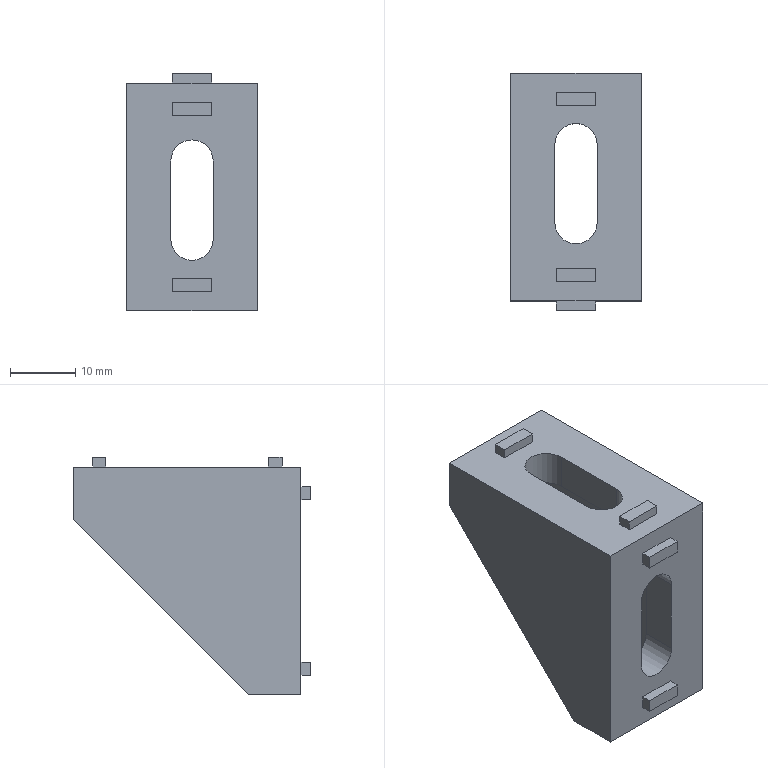Part | STEP file | 30×30 aluminium angle | 1 solid | 41 faces | box 20 x 36.5 x 36.5 mm | volume 8979 mm3 | plane 36 | cylinder 5 | commonest cylinder face diameters 6.5 x5